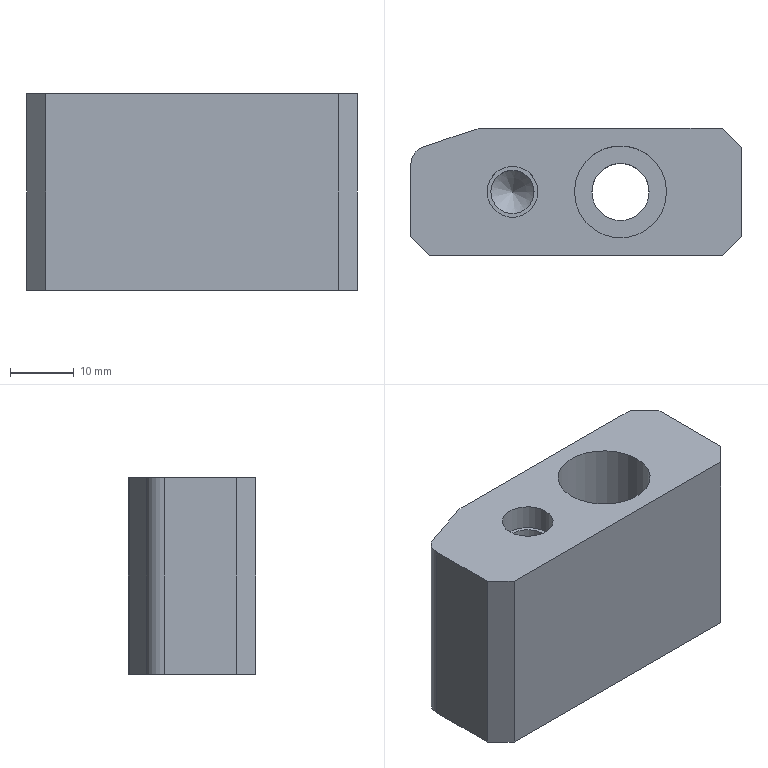Part | NX | features DIE-44 2 | 1 solid | 19 faces | box 52 x 20 x 31 mm | volume 27082 mm3 | plane 12 | cylinder 6 | cone 1 | commonest cylinder face diameters 6 x2 6.806 x1 8 x1 9 x1 14.5 x1
STEP:
#1=CARTESIAN_POINT('',(3599.094,-930.622,884.716));
#2=VERTEX_POINT('',#1);
#3=CARTESIAN_POINT('',(3595.094,-930.622,884.716));
#4=DIRECTION('',(0.,0.,-1.));
#5=DIRECTION('',(1.,0.,0.));
#6=AXIS2_PLACEMENT_3D('',#3,#4,#5);
#7=CIRCLE('',#6,4.);
#8=EDGE_CURVE('',#2,#2,#7,.T.);
#9=ORIENTED_EDGE('',*,*,#8,.T.);
#10=EDGE_LOOP('',(#9));
#11=FACE_BOUND('',#10,.T.);
#12=CARTESIAN_POINT('',(3619.344,-930.622,884.716));
#13=VERTEX_POINT('',#12);
#14=CARTESIAN_POINT('',(3612.094,-930.622,884.716));
#15=DIRECTION('',(0.,0.,1.));
#16=DIRECTION('',(1.,0.,0.));
#17=AXIS2_PLACEMENT_3D('',#14,#15,#16);
#18=CIRCLE('',#17,7.25);
#19=EDGE_CURVE('',#13,#13,#18,.T.);
#20=ORIENTED_EDGE('',*,*,#19,.F.);
#21=EDGE_LOOP('',(#20));
#22=FACE_BOUND('',#21,.T.);
#23=CARTESIAN_POINT('',(3589.375,-920.776,884.716));
#24=VERTEX_POINT('',#23);
#25=CARTESIAN_POINT('',(3581.145,-923.519,884.716));
#26=VERTEX_POINT('',#25);
#27=CARTESIAN_POINT('',(3524.968,-942.245,884.716));
#28=DIRECTION('',(0.9487,0.3162,0.));
#29=VECTOR('',#28,1000.);
#30=LINE('',#27,#29);
#31=EDGE_CURVE('',#24,#26,#30,.F.);
#32=ORIENTED_EDGE('',*,*,#31,.T.);
#33=CARTESIAN_POINT('',(3579.094,-926.365,884.716));
#34=VERTEX_POINT('',#33);
#35=CARTESIAN_POINT('',(3582.094,-926.365,884.716));
#36=DIRECTION('',(0.,0.,1.));
#37=DIRECTION('',(1.,0.,0.));
#38=AXIS2_PLACEMENT_3D('',#35,#36,#37);
#39=CIRCLE('',#38,3.);
#40=EDGE_CURVE('',#26,#34,#39,.T.);
#41=ORIENTED_EDGE('',*,*,#40,.T.);
#42=CARTESIAN_POINT('',(3579.094,-937.622,884.716));
#43=VERTEX_POINT('',#42);
#44=CARTESIAN_POINT('',(3579.094,-930.622,884.716));
#45=DIRECTION('',(0.,1.,0.));
#46=VECTOR('',#45,1000.);
#47=LINE('',#44,#46);
#48=EDGE_CURVE('',#43,#34,#47,.T.);
#49=ORIENTED_EDGE('',*,*,#48,.F.);
#50=CARTESIAN_POINT('',(3582.094,-940.622,884.716));
#51=VERTEX_POINT('',#50);
#52=CARTESIAN_POINT('',(3583.094,-941.622,884.716));
#53=DIRECTION('',(-0.7071,0.7071,0.));
#54=VECTOR('',#53,1000.);
#55=LINE('',#52,#54);
#56=EDGE_CURVE('',#43,#51,#55,.F.);
#57=ORIENTED_EDGE('',*,*,#56,.T.);
#58=CARTESIAN_POINT('',(3628.094,-940.622,884.716));
#59=VERTEX_POINT('',#58);
#60=CARTESIAN_POINT('',(3521.094,-940.622,884.716));
#61=DIRECTION('',(-1.,0.,0.));
#62=VECTOR('',#61,1000.);
#63=LINE('',#60,#62);
#64=EDGE_CURVE('',#59,#51,#63,.T.);
#65=ORIENTED_EDGE('',*,*,#64,.F.);
#66=CARTESIAN_POINT('',(3631.094,-937.622,884.716));
#67=VERTEX_POINT('',#66);
#68=CARTESIAN_POINT('',(3579.594,-989.122,884.716));
#69=DIRECTION('',(-0.7071,-0.7071,0.));
#70=VECTOR('',#69,1000.);
#71=LINE('',#68,#70);
#72=EDGE_CURVE('',#59,#67,#71,.F.);
#73=ORIENTED_EDGE('',*,*,#72,.T.);
#74=CARTESIAN_POINT('',(3631.094,-923.622,884.716));
#75=VERTEX_POINT('',#74);
#76=CARTESIAN_POINT('',(3631.094,-930.622,884.716));
#77=DIRECTION('',(0.,-1.,0.));
#78=VECTOR('',#77,1000.);
#79=LINE('',#76,#78);
#80=EDGE_CURVE('',#75,#67,#79,.T.);
#81=ORIENTED_EDGE('',*,*,#80,.F.);
#82=CARTESIAN_POINT('',(3628.094,-920.622,884.716));
#83=VERTEX_POINT('',#82);
#84=CARTESIAN_POINT('',(3579.594,-872.122,884.716));
#85=DIRECTION('',(0.7071,-0.7071,0.));
#86=VECTOR('',#85,1000.);
#87=LINE('',#84,#86);
#88=EDGE_CURVE('',#75,#83,#87,.F.);
#89=ORIENTED_EDGE('',*,*,#88,.T.);
#90=CARTESIAN_POINT('',(3590.324,-920.622,884.716));
#91=VERTEX_POINT('',#90);
#92=CARTESIAN_POINT('',(3521.094,-920.622,884.716));
#93=DIRECTION('',(1.,0.,0.));
#94=VECTOR('',#93,1000.);
#95=LINE('',#92,#94);
#96=EDGE_CURVE('',#91,#83,#95,.T.);
#97=ORIENTED_EDGE('',*,*,#96,.F.);
#98=CARTESIAN_POINT('',(3590.324,-923.622,884.716));
#99=DIRECTION('',(0.,0.,1.));
#100=DIRECTION('',(1.,0.,0.));
#101=AXIS2_PLACEMENT_3D('',#98,#99,#100);
#102=CIRCLE('',#101,3.);
#103=EDGE_CURVE('',#91,#24,#102,.T.);
#104=ORIENTED_EDGE('',*,*,#103,.T.);
#105=EDGE_LOOP('',(#32,#41,#49,#57,#65,#73,#81,#89,#97,#104));
#106=FACE_BOUND('',#105,.T.);
#107=CARTESIAN_POINT('',(3521.094,-930.622,884.716));
#108=DIRECTION('',(0.,0.,1.));
#109=DIRECTION('',(1.,0.,0.));
#110=AXIS2_PLACEMENT_3D('',#107,#108,#109);
#111=PLANE('',#110);
#112=ADVANCED_FACE('',(#11,#22,#106),#111,.T.);
#113=CARTESIAN_POINT('',(3582.094,-940.622,853.716));
#114=VERTEX_POINT('',#113);
#115=CARTESIAN_POINT('',(3628.094,-940.622,853.716));
#116=VERTEX_POINT('',#115);
#117=CARTESIAN_POINT('',(3521.094,-940.622,853.716));
#118=DIRECTION('',(1.,0.,0.));
#119=VECTOR('',#118,1000.);
#120=LINE('',#117,#119);
#121=EDGE_CURVE('',#114,#116,#120,.T.);
#122=ORIENTED_EDGE('',*,*,#121,.T.);
#123=CARTESIAN_POINT('',(3628.094,-940.622,841.716));
#124=DIRECTION('',(0.,0.,-1.));
#125=VECTOR('',#124,1000.);
#126=LINE('',#123,#125);
#127=EDGE_CURVE('',#116,#59,#126,.F.);
#128=ORIENTED_EDGE('',*,*,#127,.T.);
#129=ORIENTED_EDGE('',*,*,#64,.T.);
#130=CARTESIAN_POINT('',(3582.094,-940.622,841.716));
#131=DIRECTION('',(0.,0.,-1.));
#132=VECTOR('',#131,1000.);
#133=LINE('',#130,#132);
#134=EDGE_CURVE('',#51,#114,#133,.T.);
#135=ORIENTED_EDGE('',*,*,#134,.T.);
#136=EDGE_LOOP('',(#122,#128,#129,#135));
#137=FACE_BOUND('',#136,.T.);
#138=CARTESIAN_POINT('',(3521.094,-940.622,841.716));
#139=DIRECTION('',(0.,-1.,0.));
#140=DIRECTION('',(0.,0.,-1.));
#141=AXIS2_PLACEMENT_3D('',#138,#139,#140);
#142=PLANE('',#141);
#143=ADVANCED_FACE('',(#137),#142,.T.);
#144=ORIENTED_EDGE('',*,*,#48,.T.);
#145=CARTESIAN_POINT('',(3579.094,-926.365,853.716));
#146=VERTEX_POINT('',#145);
#147=CARTESIAN_POINT('',(3579.094,-926.365,841.716));
#148=DIRECTION('',(0.,0.,1.));
#149=VECTOR('',#148,1000.);
#150=LINE('',#147,#149);
#151=EDGE_CURVE('',#34,#146,#150,.F.);
#152=ORIENTED_EDGE('',*,*,#151,.T.);
#153=CARTESIAN_POINT('',(3579.094,-937.622,853.716));
#154=VERTEX_POINT('',#153);
#155=CARTESIAN_POINT('',(3579.094,-930.622,853.716));
#156=DIRECTION('',(0.,-1.,0.));
#157=VECTOR('',#156,1000.);
#158=LINE('',#155,#157);
#159=EDGE_CURVE('',#146,#154,#158,.T.);
#160=ORIENTED_EDGE('',*,*,#159,.T.);
#161=CARTESIAN_POINT('',(3579.094,-937.622,841.716));
#162=DIRECTION('',(0.,0.,1.));
#163=VECTOR('',#162,1000.);
#164=LINE('',#161,#163);
#165=EDGE_CURVE('',#154,#43,#164,.T.);
#166=ORIENTED_EDGE('',*,*,#165,.T.);
#167=EDGE_LOOP('',(#144,#152,#160,#166));
#168=FACE_BOUND('',#167,.T.);
#169=CARTESIAN_POINT('',(3579.094,-930.622,841.716));
#170=DIRECTION('',(-1.,0.,0.));
#171=DIRECTION('',(0.,0.,1.));
#172=AXIS2_PLACEMENT_3D('',#169,#170,#171);
#173=PLANE('',#172);
#174=ADVANCED_FACE('',(#168),#173,.T.);
#175=CARTESIAN_POINT('',(3628.094,-920.622,853.716));
#176=VERTEX_POINT('',#175);
#177=CARTESIAN_POINT('',(3590.324,-920.622,853.716));
#178=VERTEX_POINT('',#177);
#179=CARTESIAN_POINT('',(3521.094,-920.622,853.716));
#180=DIRECTION('',(-1.,0.,0.));
#181=VECTOR('',#180,1000.);
#182=LINE('',#179,#181);
#183=EDGE_CURVE('',#176,#178,#182,.T.);
#184=ORIENTED_EDGE('',*,*,#183,.T.);
#185=CARTESIAN_POINT('',(3590.324,-920.622,841.716));
#186=DIRECTION('',(0.,0.,-1.));
#187=VECTOR('',#186,1000.);
#188=LINE('',#185,#187);
#189=EDGE_CURVE('',#178,#91,#188,.F.);
#190=ORIENTED_EDGE('',*,*,#189,.T.);
#191=ORIENTED_EDGE('',*,*,#96,.T.);
#192=CARTESIAN_POINT('',(3628.094,-920.622,841.716));
#193=DIRECTION('',(0.,0.,1.));
#194=VECTOR('',#193,1000.);
#195=LINE('',#192,#194);
#196=EDGE_CURVE('',#83,#176,#195,.F.);
#197=ORIENTED_EDGE('',*,*,#196,.T.);
#198=EDGE_LOOP('',(#184,#190,#191,#197));
#199=FACE_BOUND('',#198,.T.);
#200=CARTESIAN_POINT('',(3521.094,-920.622,841.716));
#201=DIRECTION('',(0.,1.,0.));
#202=DIRECTION('',(0.,0.,1.));
#203=AXIS2_PLACEMENT_3D('',#200,#201,#202);
#204=PLANE('',#203);
#205=ADVANCED_FACE('',(#199),#204,.T.);
#206=CARTESIAN_POINT('',(3607.594,-930.622,853.716));
#207=VERTEX_POINT('',#206);
#208=CARTESIAN_POINT('',(3612.094,-930.622,853.716));
#209=DIRECTION('',(0.,0.,-1.));
#210=DIRECTION('',(-1.,0.,0.));
#211=AXIS2_PLACEMENT_3D('',#208,#209,#210);
#212=CIRCLE('',#211,4.5);
#213=EDGE_CURVE('',#207,#207,#212,.T.);
#214=ORIENTED_EDGE('',*,*,#213,.F.);
#215=EDGE_LOOP('',(#214));
#216=FACE_BOUND('',#215,.T.);
#217=ORIENTED_EDGE('',*,*,#159,.F.);
#218=CARTESIAN_POINT('',(3581.145,-923.519,853.716));
#219=VERTEX_POINT('',#218);
#220=CARTESIAN_POINT('',(3582.094,-926.365,853.716));
#221=DIRECTION('',(0.,0.,-1.));
#222=DIRECTION('',(-1.,0.,0.));
#223=AXIS2_PLACEMENT_3D('',#220,#221,#222);
#224=CIRCLE('',#223,3.);
#225=EDGE_CURVE('',#146,#219,#224,.T.);
#226=ORIENTED_EDGE('',*,*,#225,.T.);
#227=CARTESIAN_POINT('',(3589.375,-920.776,853.716));
#228=VERTEX_POINT('',#227);
#229=CARTESIAN_POINT('',(3524.968,-942.245,853.716));
#230=DIRECTION('',(-0.9487,-0.3162,0.));
#231=VECTOR('',#230,1000.);
#232=LINE('',#229,#231);
#233=EDGE_CURVE('',#219,#228,#232,.F.);
#234=ORIENTED_EDGE('',*,*,#233,.T.);
#235=CARTESIAN_POINT('',(3590.324,-923.622,853.716));
#236=DIRECTION('',(0.,0.,-1.));
#237=DIRECTION('',(-1.,0.,0.));
#238=AXIS2_PLACEMENT_3D('',#235,#236,#237);
#239=CIRCLE('',#238,3.);
#240=EDGE_CURVE('',#228,#178,#239,.T.);
#241=ORIENTED_EDGE('',*,*,#240,.T.);
#242=ORIENTED_EDGE('',*,*,#183,.F.);
#243=CARTESIAN_POINT('',(3631.094,-923.622,853.716));
#244=VERTEX_POINT('',#243);
#245=CARTESIAN_POINT('',(3579.594,-872.122,853.716));
#246=DIRECTION('',(-0.7071,0.7071,0.));
#247=VECTOR('',#246,1000.);
#248=LINE('',#245,#247);
#249=EDGE_CURVE('',#176,#244,#248,.F.);
#250=ORIENTED_EDGE('',*,*,#249,.T.);
#251=CARTESIAN_POINT('',(3631.094,-937.622,853.716));
#252=VERTEX_POINT('',#251);
#253=CARTESIAN_POINT('',(3631.094,-930.622,853.716));
#254=DIRECTION('',(0.,1.,0.));
#255=VECTOR('',#254,1000.);
#256=LINE('',#253,#255);
#257=EDGE_CURVE('',#252,#244,#256,.T.);
#258=ORIENTED_EDGE('',*,*,#257,.F.);
#259=CARTESIAN_POINT('',(3579.594,-989.122,853.716));
#260=DIRECTION('',(0.7071,0.7071,0.));
#261=VECTOR('',#260,1000.);
#262=LINE('',#259,#261);
#263=EDGE_CURVE('',#252,#116,#262,.F.);
#264=ORIENTED_EDGE('',*,*,#263,.T.);
#265=ORIENTED_EDGE('',*,*,#121,.F.);
#266=CARTESIAN_POINT('',(3546.594,-905.122,853.716));
#267=DIRECTION('',(0.7071,-0.7071,0.));
#268=VECTOR('',#267,1000.);
#269=LINE('',#266,#268);
#270=EDGE_CURVE('',#114,#154,#269,.F.);
#271=ORIENTED_EDGE('',*,*,#270,.T.);
#272=EDGE_LOOP('',(#217,#226,#234,#241,#242,#250,#258,#264,#265,#271));
#273=FACE_BOUND('',#272,.T.);
#274=CARTESIAN_POINT('',(3521.094,-930.622,853.716));
#275=DIRECTION('',(0.,0.,-1.));
#276=DIRECTION('',(-1.,0.,0.));
#277=AXIS2_PLACEMENT_3D('',#274,#275,#276);
#278=PLANE('',#277);
#279=ADVANCED_FACE('',(#216,#273),#278,.T.);
#280=ORIENTED_EDGE('',*,*,#257,.T.);
#281=CARTESIAN_POINT('',(3631.094,-923.622,841.716));
#282=DIRECTION('',(0.,0.,-1.));
#283=VECTOR('',#282,1000.);
#284=LINE('',#281,#283);
#285=EDGE_CURVE('',#244,#75,#284,.F.);
#286=ORIENTED_EDGE('',*,*,#285,.T.);
#287=ORIENTED_EDGE('',*,*,#80,.T.);
#288=CARTESIAN_POINT('',(3631.094,-937.622,841.716));
#289=DIRECTION('',(0.,0.,1.));
#290=VECTOR('',#289,1000.);
#291=LINE('',#288,#290);
#292=EDGE_CURVE('',#67,#252,#291,.F.);
#293=ORIENTED_EDGE('',*,*,#292,.T.);
#294=EDGE_LOOP('',(#280,#286,#287,#293));
#295=FACE_BOUND('',#294,.T.);
#296=CARTESIAN_POINT('',(3631.094,-930.622,841.716));
#297=DIRECTION('',(1.,0.,0.));
#298=DIRECTION('',(0.,0.,-1.));
#299=AXIS2_PLACEMENT_3D('',#296,#297,#298);
#300=PLANE('',#299);
#301=ADVANCED_FACE('',(#295),#300,.T.);
#302=ORIENTED_EDGE('',*,*,#263,.F.);
#303=ORIENTED_EDGE('',*,*,#292,.F.);
#304=ORIENTED_EDGE('',*,*,#72,.F.);
#305=ORIENTED_EDGE('',*,*,#127,.F.);
#306=EDGE_LOOP('',(#302,#303,#304,#305));
#307=FACE_BOUND('',#306,.T.);
#308=CARTESIAN_POINT('',(3628.094,-940.622,841.716));
#309=DIRECTION('',(-0.7071,0.7071,0.));
#310=DIRECTION('',(-0.7071,-0.7071,0.));
#311=AXIS2_PLACEMENT_3D('',#308,#309,#310);
#312=PLANE('',#311);
#313=ADVANCED_FACE('',(#307),#312,.F.);
#314=ORIENTED_EDGE('',*,*,#270,.F.);
#315=ORIENTED_EDGE('',*,*,#134,.F.);
#316=ORIENTED_EDGE('',*,*,#56,.F.);
#317=ORIENTED_EDGE('',*,*,#165,.F.);
#318=EDGE_LOOP('',(#314,#315,#316,#317));
#319=FACE_BOUND('',#318,.T.);
#320=CARTESIAN_POINT('',(3579.094,-937.622,841.716));
#321=DIRECTION('',(0.7071,0.7071,0.));
#322=DIRECTION('',(0.,0.,1.));
#323=AXIS2_PLACEMENT_3D('',#320,#321,#322);
#324=PLANE('',#323);
#325=ADVANCED_FACE('',(#319),#324,.F.);
#326=ORIENTED_EDGE('',*,*,#249,.F.);
#327=ORIENTED_EDGE('',*,*,#196,.F.);
#328=ORIENTED_EDGE('',*,*,#88,.F.);
#329=ORIENTED_EDGE('',*,*,#285,.F.);
#330=EDGE_LOOP('',(#326,#327,#328,#329));
#331=FACE_BOUND('',#330,.T.);
#332=CARTESIAN_POINT('',(3631.094,-923.622,841.716));
#333=DIRECTION('',(-0.7071,-0.7071,0.));
#334=DIRECTION('',(0.7071,-0.7071,0.));
#335=AXIS2_PLACEMENT_3D('',#332,#333,#334);
#336=PLANE('',#335);
#337=ADVANCED_FACE('',(#331),#336,.F.);
#338=ORIENTED_EDGE('',*,*,#233,.F.);
#339=CARTESIAN_POINT('',(3581.145,-923.519,841.716));
#340=DIRECTION('',(0.,0.,-1.));
#341=VECTOR('',#340,1000.);
#342=LINE('',#339,#341);
#343=EDGE_CURVE('',#219,#26,#342,.F.);
#344=ORIENTED_EDGE('',*,*,#343,.T.);
#345=ORIENTED_EDGE('',*,*,#31,.F.);
#346=CARTESIAN_POINT('',(3589.375,-920.776,841.716));
#347=DIRECTION('',(0.,0.,1.));
#348=VECTOR('',#347,1000.);
#349=LINE('',#346,#348);
#350=EDGE_CURVE('',#24,#228,#349,.F.);
#351=ORIENTED_EDGE('',*,*,#350,.T.);
#352=EDGE_LOOP('',(#338,#344,#345,#351));
#353=FACE_BOUND('',#352,.T.);
#354=CARTESIAN_POINT('',(3585.568,-922.045,841.716));
#355=DIRECTION('',(0.3162,-0.9487,0.));
#356=DIRECTION('',(0.,0.,1.));
#357=AXIS2_PLACEMENT_3D('',#354,#355,#356);
#358=PLANE('',#357);
#359=ADVANCED_FACE('',(#353),#358,.F.);
#360=ORIENTED_EDGE('',*,*,#40,.F.);
#361=ORIENTED_EDGE('',*,*,#343,.F.);
#362=ORIENTED_EDGE('',*,*,#225,.F.);
#363=ORIENTED_EDGE('',*,*,#151,.F.);
#364=EDGE_LOOP('',(#360,#361,#362,#363));
#365=FACE_BOUND('',#364,.T.);
#366=CARTESIAN_POINT('',(3582.094,-926.365,841.716));
#367=DIRECTION('',(0.,0.,1.));
#368=DIRECTION('',(1.,0.,0.));
#369=AXIS2_PLACEMENT_3D('',#366,#367,#368);
#370=CYLINDRICAL_SURFACE('',#369,3.);
#371=ADVANCED_FACE('',(#365),#370,.T.);
#372=ORIENTED_EDGE('',*,*,#240,.F.);
#373=ORIENTED_EDGE('',*,*,#350,.F.);
#374=ORIENTED_EDGE('',*,*,#103,.F.);
#375=ORIENTED_EDGE('',*,*,#189,.F.);
#376=EDGE_LOOP('',(#372,#373,#374,#375));
#377=FACE_BOUND('',#376,.T.);
#378=CARTESIAN_POINT('',(3590.324,-923.622,841.716));
#379=DIRECTION('',(0.,0.,-1.));
#380=DIRECTION('',(-1.,0.,0.));
#381=AXIS2_PLACEMENT_3D('',#378,#379,#380);
#382=CYLINDRICAL_SURFACE('',#381,3.);
#383=ADVANCED_FACE('',(#377),#382,.T.);
#384=ORIENTED_EDGE('',*,*,#213,.T.);
#385=EDGE_LOOP('',(#384));
#386=FACE_BOUND('',#385,.T.);
#387=CARTESIAN_POINT('',(3616.594,-930.622,871.716));
#388=VERTEX_POINT('',#387);
#389=CARTESIAN_POINT('',(3612.094,-930.622,871.716));
#390=DIRECTION('',(0.,0.,1.));
#391=DIRECTION('',(1.,0.,0.));
#392=AXIS2_PLACEMENT_3D('',#389,#390,#391);
#393=CIRCLE('',#392,4.5);
#394=EDGE_CURVE('',#388,#388,#393,.T.);
#395=ORIENTED_EDGE('',*,*,#394,.T.);
#396=EDGE_LOOP('',(#395));
#397=FACE_BOUND('',#396,.T.);
#398=CARTESIAN_POINT('',(3612.094,-930.622,845.716));
#399=DIRECTION('',(0.,0.,1.));
#400=DIRECTION('',(1.,0.,0.));
#401=AXIS2_PLACEMENT_3D('',#398,#399,#400);
#402=CYLINDRICAL_SURFACE('',#401,4.5);
#403=ADVANCED_FACE('',(#386,#397),#402,.F.);
#404=ORIENTED_EDGE('',*,*,#19,.T.);
#405=EDGE_LOOP('',(#404));
#406=FACE_BOUND('',#405,.T.);
#407=CARTESIAN_POINT('',(3619.344,-930.622,871.716));
#408=VERTEX_POINT('',#407);
#409=CARTESIAN_POINT('',(3612.094,-930.622,871.716));
#410=DIRECTION('',(0.,0.,1.));
#411=DIRECTION('',(1.,0.,0.));
#412=AXIS2_PLACEMENT_3D('',#409,#410,#411);
#413=CIRCLE('',#412,7.25);
#414=EDGE_CURVE('',#408,#408,#413,.F.);
#415=ORIENTED_EDGE('',*,*,#414,.T.);
#416=EDGE_LOOP('',(#415));
#417=FACE_BOUND('',#416,.T.);
#418=CARTESIAN_POINT('',(3612.094,-930.622,871.716));
#419=DIRECTION('',(0.,0.,1.));
#420=DIRECTION('',(1.,0.,0.));
#421=AXIS2_PLACEMENT_3D('',#418,#419,#420);
#422=CYLINDRICAL_SURFACE('',#421,7.25);
#423=ADVANCED_FACE('',(#406,#417),#422,.F.);
#424=ORIENTED_EDGE('',*,*,#394,.F.);
#425=EDGE_LOOP('',(#424));
#426=FACE_BOUND('',#425,.T.);
#427=ORIENTED_EDGE('',*,*,#414,.F.);
#428=EDGE_LOOP('',(#427));
#429=FACE_BOUND('',#428,.T.);
#430=CARTESIAN_POINT('',(3612.094,-930.622,871.716));
#431=DIRECTION('',(0.,0.,1.));
#432=DIRECTION('',(1.,0.,0.));
#433=AXIS2_PLACEMENT_3D('',#430,#431,#432);
#434=PLANE('',#433);
#435=ADVANCED_FACE('',(#426,#429),#434,.T.);
#436=CARTESIAN_POINT('',(3591.691,-930.622,880.716));
#437=VERTEX_POINT('',#436);
#438=CARTESIAN_POINT('',(3595.094,-930.622,880.716));
#439=DIRECTION('',(0.,0.,-1.));
#440=DIRECTION('',(-1.,0.,0.));
#441=AXIS2_PLACEMENT_3D('',#438,#439,#440);
#442=CIRCLE('',#441,3.403);
#443=EDGE_CURVE('',#437,#437,#442,.T.);
#444=ORIENTED_EDGE('',*,*,#443,.F.);
#445=EDGE_LOOP('',(#444));
#446=FACE_BOUND('',#445,.T.);
#447=CARTESIAN_POINT('',(3591.691,-930.622,864.716));
#448=VERTEX_POINT('',#447);
#449=CARTESIAN_POINT('',(3595.094,-930.622,864.716));
#450=DIRECTION('',(0.,0.,-1.));
#451=DIRECTION('',(-1.,0.,0.));
#452=AXIS2_PLACEMENT_3D('',#449,#450,#451);
#453=CIRCLE('',#452,3.403);
#454=EDGE_CURVE('',#448,#448,#453,.T.);
#455=ORIENTED_EDGE('',*,*,#454,.T.);
#456=EDGE_LOOP('',(#455));
#457=FACE_BOUND('',#456,.T.);
#458=CARTESIAN_POINT('',(3595.094,-930.622,889.716));
#459=DIRECTION('',(0.,0.,-1.));
#460=DIRECTION('',(1.,0.,0.));
#461=AXIS2_PLACEMENT_3D('',#458,#459,#460);
#462=CYLINDRICAL_SURFACE('',#461,3.403);
#463=ADVANCED_FACE('',(#446,#457),#462,.F.);
#464=CARTESIAN_POINT('',(3595.094,-930.622,861.313));
#465=VERTEX_POINT('',#464);
#466=VERTEX_LOOP('',#465);
#467=FACE_BOUND('',#466,.T.);
#468=ORIENTED_EDGE('',*,*,#454,.F.);
#469=EDGE_LOOP('',(#468));
#470=FACE_BOUND('',#469,.T.);
#471=CARTESIAN_POINT('',(3595.094,-930.622,864.716));
#472=DIRECTION('',(0.,0.,1.));
#473=DIRECTION('',(1.,0.,0.));
#474=AXIS2_PLACEMENT_3D('',#471,#472,#473);
#475=CONICAL_SURFACE('',#474,3.403,0.7854);
#476=ADVANCED_FACE('',(#467,#470),#475,.F.);
#477=ORIENTED_EDGE('',*,*,#443,.T.);
#478=EDGE_LOOP('',(#477));
#479=FACE_BOUND('',#478,.T.);
#480=CARTESIAN_POINT('',(3599.094,-930.622,880.716));
#481=VERTEX_POINT('',#480);
#482=CARTESIAN_POINT('',(3595.094,-930.622,880.716));
#483=DIRECTION('',(0.,0.,1.));
#484=DIRECTION('',(1.,0.,0.));
#485=AXIS2_PLACEMENT_3D('',#482,#483,#484);
#486=CIRCLE('',#485,4.);
#487=EDGE_CURVE('',#481,#481,#486,.F.);
#488=ORIENTED_EDGE('',*,*,#487,.F.);
#489=EDGE_LOOP('',(#488));
#490=FACE_BOUND('',#489,.T.);
#491=CARTESIAN_POINT('',(3595.094,-930.622,880.716));
#492=DIRECTION('',(0.,0.,-1.));
#493=DIRECTION('',(-1.,0.,0.));
#494=AXIS2_PLACEMENT_3D('',#491,#492,#493);
#495=PLANE('',#494);
#496=ADVANCED_FACE('',(#479,#490),#495,.F.);
#497=ORIENTED_EDGE('',*,*,#487,.T.);
#498=EDGE_LOOP('',(#497));
#499=FACE_BOUND('',#498,.T.);
#500=ORIENTED_EDGE('',*,*,#8,.F.);
#501=EDGE_LOOP('',(#500));
#502=FACE_BOUND('',#501,.T.);
#503=CARTESIAN_POINT('',(3595.094,-930.622,884.716));
#504=DIRECTION('',(0.,0.,-1.));
#505=DIRECTION('',(1.,0.,0.));
#506=AXIS2_PLACEMENT_3D('',#503,#504,#505);
#507=CYLINDRICAL_SURFACE('',#506,4.);
#508=ADVANCED_FACE('',(#499,#502),#507,.F.);
#509=CLOSED_SHELL('',(#112,#143,#174,#205,#279,#301,#313,#325,#337,#359,#371,#383,#403,#423,#435,#463,#476,#496,#508));
#510=MANIFOLD_SOLID_BREP('',#509);
#511=(LENGTH_UNIT()NAMED_UNIT(*)SI_UNIT(.MILLI.,.METRE.));
#512=UNCERTAINTY_MEASURE_WITH_UNIT(LENGTH_MEASURE(0.00001),#511,'','');
#513=(NAMED_UNIT(*)PLANE_ANGLE_UNIT()SI_UNIT($,.RADIAN.));
#514=(NAMED_UNIT(*)SI_UNIT($,.STERADIAN.)SOLID_ANGLE_UNIT());
#515=(GEOMETRIC_REPRESENTATION_CONTEXT(3)GLOBAL_UNCERTAINTY_ASSIGNED_CONTEXT((#512))GLOBAL_UNIT_ASSIGNED_CONTEXT((#511,#513,#514))REPRESENTATION_CONTEXT('',''));
#516=ADVANCED_BREP_SHAPE_REPRESENTATION('',(#510),#515);